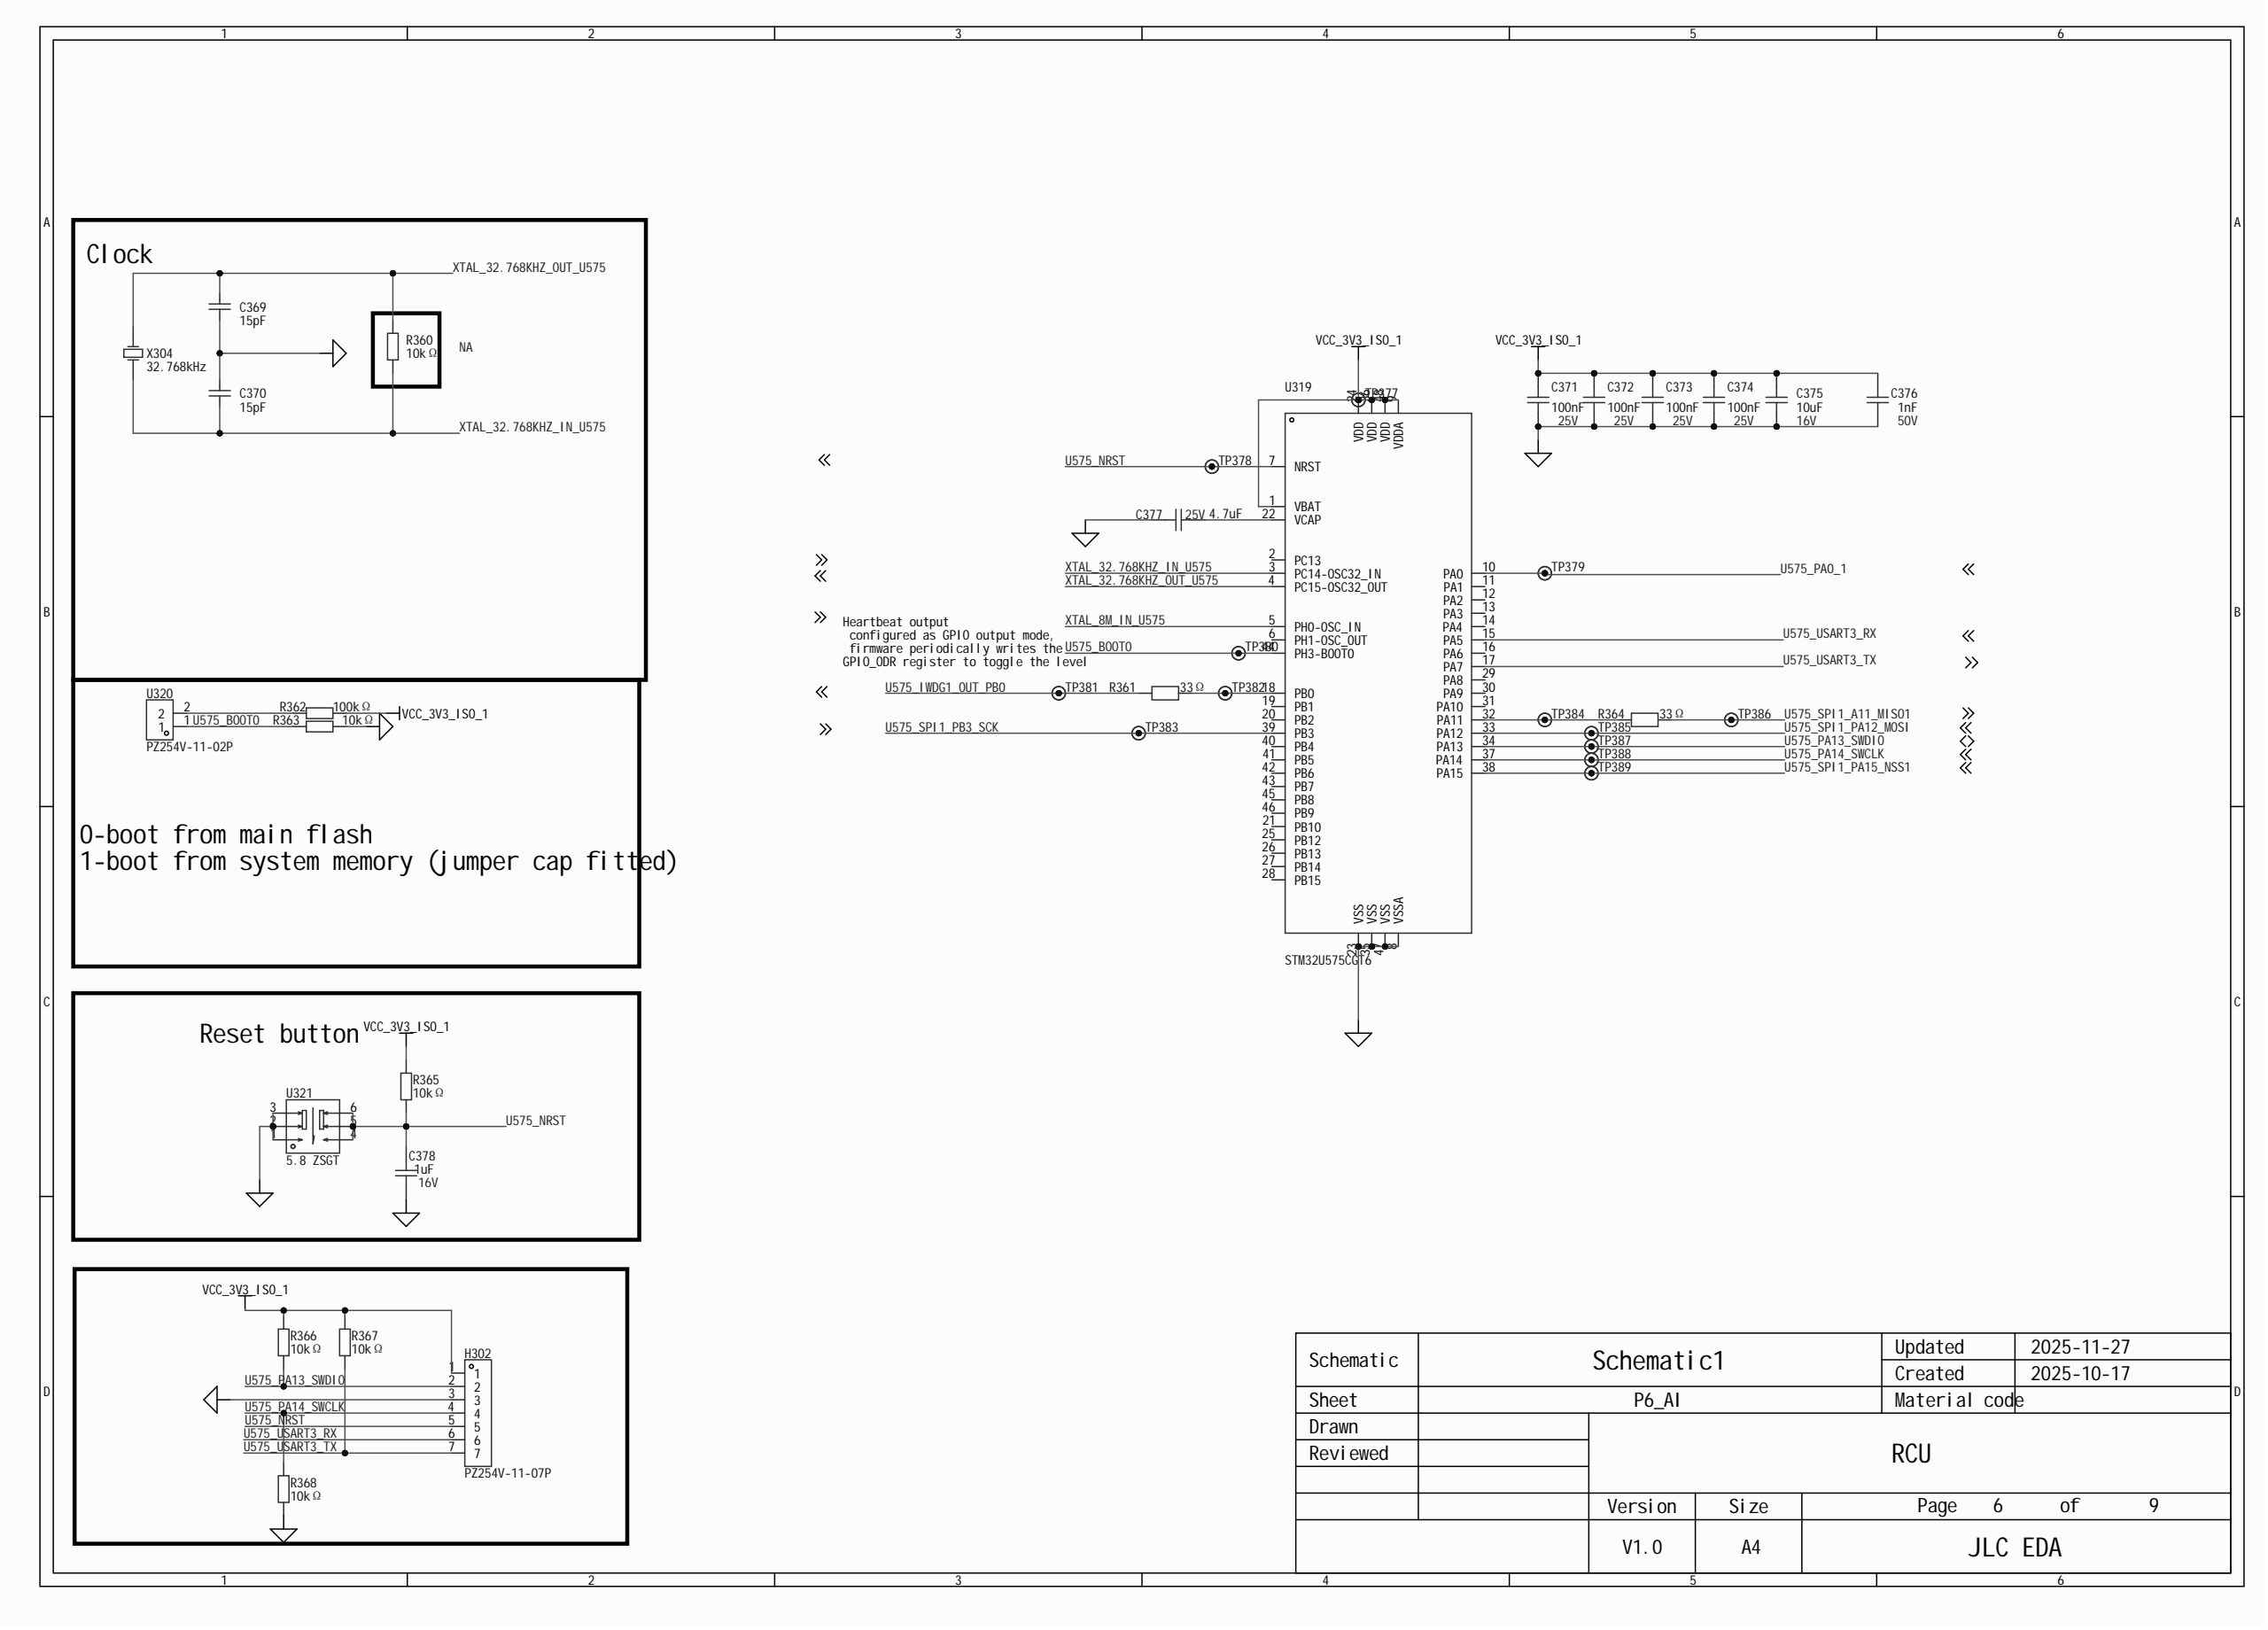Circuit board | Altium Designer | 424 parts | 202 nets | one sheet of the schematic
Parts on this sheet (reference | value | footprint):
C369 | 15pF | C0402
C370 | 15pF | C0402
C371 | 100nF | C0603
C372 | 100nF | C0603
C373 | 100nF | C0603
C374 | 100nF | C0603
C375 | 10uF | C0805
C376 | 1nF | C0603
C377 | 4.7uF | C0603
C378 | 1uF | C0603
H302 | PZ254V-11-07P | HDR-TH_7P-P2.54-V-M
R360 | 10kΩ | R0402
R361 | 33Ω | R0603
R362 | 100kΩ | R0603
R363 | 10kΩ | R0603
R364 | 33Ω | R0603
R365 | 10kΩ | R0603
R366 | 10kΩ | R0603
R367 | 10kΩ | R0603
R368 | 10kΩ | R0603
TP377 | Test-Point-0.5mm
TP378 | Test-Point-0.5mm
TP379 | Test-Point-0.5mm
TP380 | Test-Point-0.5mm
TP381 | Test-Point-0.5mm
TP382 | Test-Point-0.5mm
TP383 | Test-Point-0.5mm
TP384 | Test-Point-0.5mm
TP385 | Test-Point-0.5mm
TP386 | Test-Point-0.5mm
TP387 | Test-Point-0.5mm
TP388 | Test-Point-0.5mm
TP389 | Test-Point-0.5mm
U319 | STM32U575CGT6 | LQFP-48_L7.0-W7.0-P0.50-LS9.0-TL
U320 | PZ254V-11-02P | HDR-TH_2P-P2.54-V-M
U321 | 5.8 ZSGT | SW-TH_5.8ZSGT
X304 | 32.768kHz | OSC-TH_BD3.1-P0.8-D0.3
Nets of these parts (net: part-pin ...):
XTAL_32.768KHZ_OUT_U575: C369-2 R360-2 X304-2 U319-4
XTAL_32.768KHZ_IN_U575: C370-1 R360-1 X304-1 U319-3
XTAL_8M_IN_U575: U319-5
VCC_3V3_ISO_1: C371-1 C372-1 C373-1 C374-1 C375-2 C376-2 H302-1 R362-2 R365-2 R366-2 R367-2 TP377-1 U319-1 U319-9 U319-24 U319-36 U319-48
U575_USART3_TX: H302-7 R367-1 U319-17
U575_USART3_RX: H302-6 U319-15
U575_SPI1_PB3_SCK: TP383-1 U319-39
U575_SPI1_PA15_NSS1: TP389-1 U319-38
U575_SPI1_PA12_MOSI: TP385-1 U319-33
U575_SPI1_A11_MISO1: R364-1 TP386-1
U575_PA14_SWCLK: H302-4 R368-1 TP388-1 U319-37
U575_PA13_SWDIO: H302-2 R366-1 TP387-1 U319-34
U575_PA0_1: TP379-1 U319-10
U575_NRST: C378-2 H302-5 R365-1 TP378-1 U321-4 U321-5 U321-6 U319-7
U575_IWDG1_OUT_PB0: R361-2 TP381-1
U575_BOOT0: R363-1 TP380-1 U320-1 U319-44
PGND: C369-1 C370-2 C371-2 C372-2 C373-2 C374-2 C375-1 C376-1 C377-2 C378-1 H302-3 R363-2 R368-2 U321-1 U321-2 U321-3 U319-8 U319-23 U319-35 U319-47
NetR364_2: R364-2 TP384-1 U319-32
NetR362_1: R362-1 U320-2
NetR361_1: R361-1 TP382-1 U319-18
NetC377_1: C377-1 U319-22